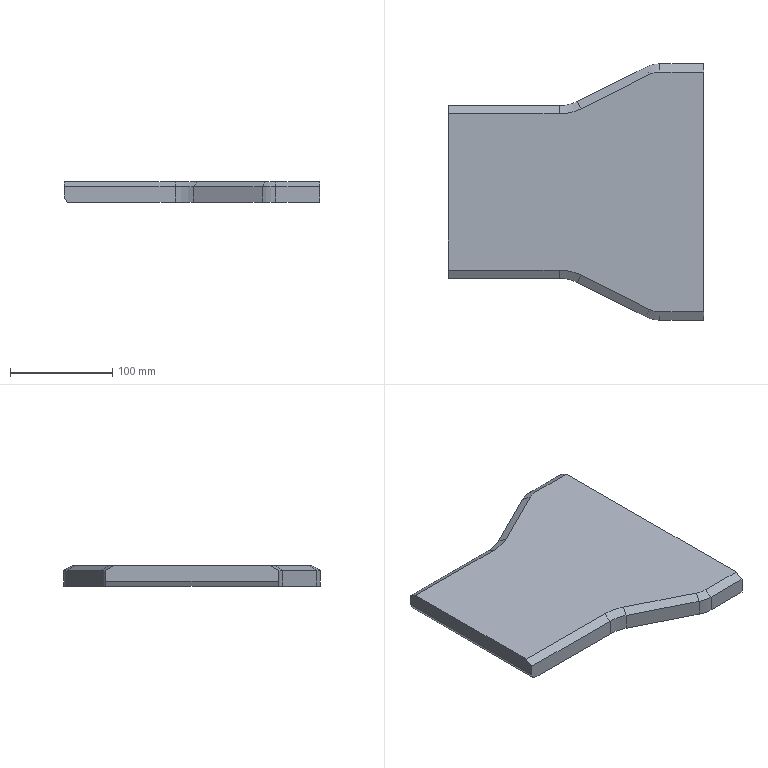Part | SolidWorks | features Chamfer 2, Extrusion 1 | 1 solid | 25 faces | box 250 x 251 x 20 mm | volume 983303 mm3 | plane 17 | cylinder 4 | cone 4 | commonest cylinder face diameters 60 x2 80 x2
STEP:
#1=CARTESIAN_POINT('',(-280.,-251.,-20.));
#2=VERTEX_POINT('',#1);
#3=CARTESIAN_POINT('',(-280.,-251.,-4.619));
#4=VERTEX_POINT('',#3);
#5=CARTESIAN_POINT('',(-280.,-251.,-20.));
#6=DIRECTION('',(0.,0.,1.));
#7=VECTOR('',#6,1000.);
#8=LINE('',#5,#7);
#9=EDGE_CURVE('',#2,#4,#8,.T.);
#10=ORIENTED_EDGE('',*,*,#9,.T.);
#11=CARTESIAN_POINT('',(-322.918,-251.,-4.619));
#12=VERTEX_POINT('',#11);
#13=CARTESIAN_POINT('',(-305.508,-251.,-4.619));
#14=DIRECTION('',(-1.,0.,0.));
#15=VECTOR('',#14,1000.);
#16=LINE('',#13,#15);
#17=EDGE_CURVE('',#4,#12,#16,.T.);
#18=ORIENTED_EDGE('',*,*,#17,.T.);
#19=CARTESIAN_POINT('',(-322.918,-251.,-20.));
#20=VERTEX_POINT('',#19);
#21=CARTESIAN_POINT('',(-322.918,-251.,-20.));
#22=DIRECTION('',(0.,0.,1.));
#23=VECTOR('',#22,1000.);
#24=LINE('',#21,#23);
#25=EDGE_CURVE('',#20,#12,#24,.T.);
#26=ORIENTED_EDGE('',*,*,#25,.F.);
#27=CARTESIAN_POINT('',(-280.,-251.,-20.));
#28=DIRECTION('',(1.,0.,0.));
#29=VECTOR('',#28,1000.);
#30=LINE('',#27,#29);
#31=EDGE_CURVE('',#20,#2,#30,.T.);
#32=ORIENTED_EDGE('',*,*,#31,.T.);
#33=EDGE_LOOP('',(#10,#18,#26,#32));
#34=FACE_OUTER_BOUND('',#33,.T.);
#35=CARTESIAN_POINT('',(-305.508,-251.,-20.));
#36=DIRECTION('',(0.,-1.,0.));
#37=DIRECTION('',(0.,0.,-1.));
#38=AXIS2_PLACEMENT_3D('',#35,#36,#37);
#39=PLANE('',#38);
#40=ADVANCED_FACE('',(#34),#39,.T.);
#41=ORIENTED_EDGE('',*,*,#25,.T.);
#42=CARTESIAN_POINT('',(-336.334,-247.833,-4.619));
#43=VERTEX_POINT('',#42);
#44=CARTESIAN_POINT('',(-322.918,-221.,-4.619));
#45=DIRECTION('',(0.,0.,-1.));
#46=DIRECTION('',(1.,0.,0.));
#47=AXIS2_PLACEMENT_3D('',#44,#45,#46);
#48=CIRCLE('',#47,30.);
#49=EDGE_CURVE('',#12,#43,#48,.T.);
#50=ORIENTED_EDGE('',*,*,#49,.T.);
#51=CARTESIAN_POINT('',(-336.334,-247.833,-20.));
#52=VERTEX_POINT('',#51);
#53=CARTESIAN_POINT('',(-336.334,-247.833,-20.));
#54=DIRECTION('',(0.,0.,1.));
#55=VECTOR('',#54,1000.);
#56=LINE('',#53,#55);
#57=EDGE_CURVE('',#52,#43,#56,.T.);
#58=ORIENTED_EDGE('',*,*,#57,.F.);
#59=CARTESIAN_POINT('',(-322.918,-221.,-20.));
#60=DIRECTION('',(0.,0.,1.));
#61=DIRECTION('',(1.,0.,0.));
#62=AXIS2_PLACEMENT_3D('',#59,#60,#61);
#63=CIRCLE('',#62,30.);
#64=EDGE_CURVE('',#52,#20,#63,.T.);
#65=ORIENTED_EDGE('',*,*,#64,.T.);
#66=EDGE_LOOP('',(#41,#50,#58,#65));
#67=FACE_OUTER_BOUND('',#66,.T.);
#68=CARTESIAN_POINT('',(-322.918,-221.,-20.));
#69=DIRECTION('',(0.,0.,1.));
#70=DIRECTION('',(1.,0.,0.));
#71=AXIS2_PLACEMENT_3D('',#68,#69,#70);
#72=CYLINDRICAL_SURFACE('',#71,30.);
#73=ADVANCED_FACE('',(#67),#72,.T.);
#74=ORIENTED_EDGE('',*,*,#57,.T.);
#75=CARTESIAN_POINT('',(-403.666,-214.167,-4.619));
#76=VERTEX_POINT('',#75);
#77=CARTESIAN_POINT('',(-403.666,-214.167,-4.619));
#78=DIRECTION('',(-0.8944,0.4472,0.));
#79=VECTOR('',#78,1000.);
#80=LINE('',#77,#79);
#81=EDGE_CURVE('',#43,#76,#80,.T.);
#82=ORIENTED_EDGE('',*,*,#81,.T.);
#83=CARTESIAN_POINT('',(-403.666,-214.167,-20.));
#84=VERTEX_POINT('',#83);
#85=CARTESIAN_POINT('',(-403.666,-214.167,-20.));
#86=DIRECTION('',(0.,0.,1.));
#87=VECTOR('',#86,1000.);
#88=LINE('',#85,#87);
#89=EDGE_CURVE('',#84,#76,#88,.T.);
#90=ORIENTED_EDGE('',*,*,#89,.F.);
#91=CARTESIAN_POINT('',(-403.666,-214.167,-20.));
#92=DIRECTION('',(0.8944,-0.4472,0.));
#93=VECTOR('',#92,1000.);
#94=LINE('',#91,#93);
#95=EDGE_CURVE('',#84,#52,#94,.T.);
#96=ORIENTED_EDGE('',*,*,#95,.T.);
#97=EDGE_LOOP('',(#74,#82,#90,#96));
#98=FACE_OUTER_BOUND('',#97,.T.);
#99=CARTESIAN_POINT('',(-403.666,-214.167,-20.));
#100=DIRECTION('',(-0.4472,-0.8944,0.));
#101=DIRECTION('',(0.8944,-0.4472,0.));
#102=AXIS2_PLACEMENT_3D('',#99,#100,#101);
#103=PLANE('',#102);
#104=ADVANCED_FACE('',(#98),#103,.T.);
#105=ORIENTED_EDGE('',*,*,#89,.T.);
#106=CARTESIAN_POINT('',(-421.554,-209.944,-4.619));
#107=VERTEX_POINT('',#106);
#108=CARTESIAN_POINT('',(-421.554,-249.944,-4.619));
#109=DIRECTION('',(0.,0.,1.));
#110=DIRECTION('',(1.,0.,0.));
#111=AXIS2_PLACEMENT_3D('',#108,#109,#110);
#112=CIRCLE('',#111,40.);
#113=EDGE_CURVE('',#76,#107,#112,.T.);
#114=ORIENTED_EDGE('',*,*,#113,.T.);
#115=CARTESIAN_POINT('',(-421.554,-209.944,-20.));
#116=VERTEX_POINT('',#115);
#117=CARTESIAN_POINT('',(-421.554,-209.944,-20.));
#118=DIRECTION('',(0.,0.,1.));
#119=VECTOR('',#118,1000.);
#120=LINE('',#117,#119);
#121=EDGE_CURVE('',#116,#107,#120,.T.);
#122=ORIENTED_EDGE('',*,*,#121,.F.);
#123=CARTESIAN_POINT('',(-421.554,-249.944,-20.));
#124=DIRECTION('',(0.,0.,-1.));
#125=DIRECTION('',(1.,0.,0.));
#126=AXIS2_PLACEMENT_3D('',#123,#124,#125);
#127=CIRCLE('',#126,40.);
#128=EDGE_CURVE('',#116,#84,#127,.T.);
#129=ORIENTED_EDGE('',*,*,#128,.T.);
#130=EDGE_LOOP('',(#105,#114,#122,#129));
#131=FACE_OUTER_BOUND('',#130,.T.);
#132=CARTESIAN_POINT('',(-421.554,-249.944,-20.));
#133=DIRECTION('',(0.,0.,1.));
#134=DIRECTION('',(1.,0.,0.));
#135=AXIS2_PLACEMENT_3D('',#132,#133,#134);
#136=CYLINDRICAL_SURFACE('',#135,40.);
#137=ADVANCED_FACE('',(#131),#136,.F.);
#138=CARTESIAN_POINT('',(-530.,-209.944,-15.));
#139=VERTEX_POINT('',#138);
#140=CARTESIAN_POINT('',(-530.,-209.944,-4.619));
#141=VERTEX_POINT('',#140);
#142=CARTESIAN_POINT('',(-530.,-209.944,-20.));
#143=DIRECTION('',(0.,0.,1.));
#144=VECTOR('',#143,1000.);
#145=LINE('',#142,#144);
#146=EDGE_CURVE('',#139,#141,#145,.T.);
#147=ORIENTED_EDGE('',*,*,#146,.F.);
#148=CARTESIAN_POINT('',(-527.113,-209.944,-20.));
#149=VERTEX_POINT('',#148);
#150=CARTESIAN_POINT('',(-500.723,-209.944,-65.708));
#151=DIRECTION('',(0.5,0.,-0.866));
#152=VECTOR('',#151,1000.);
#153=LINE('',#150,#152);
#154=EDGE_CURVE('',#139,#149,#153,.T.);
#155=ORIENTED_EDGE('',*,*,#154,.T.);
#156=CARTESIAN_POINT('',(-421.554,-209.944,-20.));
#157=DIRECTION('',(1.,0.,0.));
#158=VECTOR('',#157,1000.);
#159=LINE('',#156,#158);
#160=EDGE_CURVE('',#149,#116,#159,.T.);
#161=ORIENTED_EDGE('',*,*,#160,.T.);
#162=ORIENTED_EDGE('',*,*,#121,.T.);
#163=CARTESIAN_POINT('',(-421.554,-209.944,-4.619));
#164=DIRECTION('',(-1.,0.,0.));
#165=VECTOR('',#164,1000.);
#166=LINE('',#163,#165);
#167=EDGE_CURVE('',#107,#141,#166,.T.);
#168=ORIENTED_EDGE('',*,*,#167,.T.);
#169=EDGE_LOOP('',(#147,#155,#161,#162,#168));
#170=FACE_OUTER_BOUND('',#169,.T.);
#171=CARTESIAN_POINT('',(-421.554,-209.944,-20.));
#172=DIRECTION('',(0.,-1.,0.));
#173=DIRECTION('',(0.,0.,-1.));
#174=AXIS2_PLACEMENT_3D('',#171,#172,#173);
#175=PLANE('',#174);
#176=ADVANCED_FACE('',(#170),#175,.T.);
#177=CARTESIAN_POINT('',(-530.,-41.056,-15.));
#178=VERTEX_POINT('',#177);
#179=CARTESIAN_POINT('',(-530.,-41.056,-4.619));
#180=VERTEX_POINT('',#179);
#181=CARTESIAN_POINT('',(-530.,-41.056,-20.));
#182=DIRECTION('',(0.,0.,1.));
#183=VECTOR('',#182,1000.);
#184=LINE('',#181,#183);
#185=EDGE_CURVE('',#178,#180,#184,.T.);
#186=ORIENTED_EDGE('',*,*,#185,.F.);
#187=CARTESIAN_POINT('',(-530.,-209.944,-15.));
#188=DIRECTION('',(0.,-1.,0.));
#189=VECTOR('',#188,1000.);
#190=LINE('',#187,#189);
#191=EDGE_CURVE('',#178,#139,#190,.T.);
#192=ORIENTED_EDGE('',*,*,#191,.T.);
#193=ORIENTED_EDGE('',*,*,#146,.T.);
#194=CARTESIAN_POINT('',(-530.,-201.944,0.));
#195=VERTEX_POINT('',#194);
#196=CARTESIAN_POINT('',(-530.,-89.938,64.667));
#197=DIRECTION('',(0.,0.866,0.5));
#198=VECTOR('',#197,1000.);
#199=LINE('',#196,#198);
#200=EDGE_CURVE('',#141,#195,#199,.T.);
#201=ORIENTED_EDGE('',*,*,#200,.T.);
#202=CARTESIAN_POINT('',(-530.,-49.056,0.));
#203=VERTEX_POINT('',#202);
#204=CARTESIAN_POINT('',(-530.,-41.056,0.));
#205=DIRECTION('',(0.,-1.,0.));
#206=VECTOR('',#205,1000.);
#207=LINE('',#204,#206);
#208=EDGE_CURVE('',#203,#195,#207,.T.);
#209=ORIENTED_EDGE('',*,*,#208,.F.);
#210=CARTESIAN_POINT('',(-530.,-34.395,-8.464));
#211=DIRECTION('',(0.,0.866,-0.5));
#212=VECTOR('',#211,1000.);
#213=LINE('',#210,#212);
#214=EDGE_CURVE('',#203,#180,#213,.T.);
#215=ORIENTED_EDGE('',*,*,#214,.T.);
#216=EDGE_LOOP('',(#186,#192,#193,#201,#209,#215));
#217=FACE_OUTER_BOUND('',#216,.T.);
#218=CARTESIAN_POINT('',(-530.,-41.056,-20.));
#219=DIRECTION('',(-1.,0.,0.));
#220=DIRECTION('',(0.,0.,1.));
#221=AXIS2_PLACEMENT_3D('',#218,#219,#220);
#222=PLANE('',#221);
#223=ADVANCED_FACE('',(#217),#222,.T.);
#224=CARTESIAN_POINT('',(-421.554,-41.056,-20.));
#225=VERTEX_POINT('',#224);
#226=CARTESIAN_POINT('',(-527.113,-41.056,-20.));
#227=VERTEX_POINT('',#226);
#228=CARTESIAN_POINT('',(-530.,-41.056,-20.));
#229=DIRECTION('',(-1.,0.,0.));
#230=VECTOR('',#229,1000.);
#231=LINE('',#228,#230);
#232=EDGE_CURVE('',#225,#227,#231,.T.);
#233=ORIENTED_EDGE('',*,*,#232,.T.);
#234=CARTESIAN_POINT('',(-527.835,-41.056,-18.75));
#235=DIRECTION('',(-0.5,0.,0.866));
#236=VECTOR('',#235,1000.);
#237=LINE('',#234,#236);
#238=EDGE_CURVE('',#227,#178,#237,.T.);
#239=ORIENTED_EDGE('',*,*,#238,.T.);
#240=ORIENTED_EDGE('',*,*,#185,.T.);
#241=CARTESIAN_POINT('',(-421.554,-41.056,-4.619));
#242=VERTEX_POINT('',#241);
#243=CARTESIAN_POINT('',(-530.,-41.056,-4.619));
#244=DIRECTION('',(1.,0.,0.));
#245=VECTOR('',#244,1000.);
#246=LINE('',#243,#245);
#247=EDGE_CURVE('',#180,#242,#246,.T.);
#248=ORIENTED_EDGE('',*,*,#247,.T.);
#249=CARTESIAN_POINT('',(-421.554,-41.056,-20.));
#250=DIRECTION('',(0.,0.,1.));
#251=VECTOR('',#250,1000.);
#252=LINE('',#249,#251);
#253=EDGE_CURVE('',#225,#242,#252,.T.);
#254=ORIENTED_EDGE('',*,*,#253,.F.);
#255=EDGE_LOOP('',(#233,#239,#240,#248,#254));
#256=FACE_OUTER_BOUND('',#255,.T.);
#257=CARTESIAN_POINT('',(-530.,-41.056,-20.));
#258=DIRECTION('',(0.,1.,0.));
#259=DIRECTION('',(-1.,0.,0.));
#260=AXIS2_PLACEMENT_3D('',#257,#258,#259);
#261=PLANE('',#260);
#262=ADVANCED_FACE('',(#256),#261,.T.);
#263=ORIENTED_EDGE('',*,*,#253,.T.);
#264=CARTESIAN_POINT('',(-403.666,-36.833,-4.619));
#265=VERTEX_POINT('',#264);
#266=CARTESIAN_POINT('',(-421.554,-1.056,-4.619));
#267=DIRECTION('',(0.,0.,1.));
#268=DIRECTION('',(1.,0.,0.));
#269=AXIS2_PLACEMENT_3D('',#266,#267,#268);
#270=CIRCLE('',#269,40.);
#271=EDGE_CURVE('',#242,#265,#270,.T.);
#272=ORIENTED_EDGE('',*,*,#271,.T.);
#273=CARTESIAN_POINT('',(-403.666,-36.833,-20.));
#274=VERTEX_POINT('',#273);
#275=CARTESIAN_POINT('',(-403.666,-36.833,-20.));
#276=DIRECTION('',(0.,0.,1.));
#277=VECTOR('',#276,1000.);
#278=LINE('',#275,#277);
#279=EDGE_CURVE('',#274,#265,#278,.T.);
#280=ORIENTED_EDGE('',*,*,#279,.F.);
#281=CARTESIAN_POINT('',(-421.554,-1.056,-20.));
#282=DIRECTION('',(0.,0.,-1.));
#283=DIRECTION('',(1.,0.,0.));
#284=AXIS2_PLACEMENT_3D('',#281,#282,#283);
#285=CIRCLE('',#284,40.);
#286=EDGE_CURVE('',#274,#225,#285,.T.);
#287=ORIENTED_EDGE('',*,*,#286,.T.);
#288=EDGE_LOOP('',(#263,#272,#280,#287));
#289=FACE_OUTER_BOUND('',#288,.T.);
#290=CARTESIAN_POINT('',(-421.554,-1.056,-20.));
#291=DIRECTION('',(0.,0.,1.));
#292=DIRECTION('',(1.,0.,0.));
#293=AXIS2_PLACEMENT_3D('',#290,#291,#292);
#294=CYLINDRICAL_SURFACE('',#293,40.);
#295=ADVANCED_FACE('',(#289),#294,.F.);
#296=ORIENTED_EDGE('',*,*,#279,.T.);
#297=CARTESIAN_POINT('',(-336.334,-3.167,-4.619));
#298=VERTEX_POINT('',#297);
#299=CARTESIAN_POINT('',(-403.666,-36.833,-4.619));
#300=DIRECTION('',(0.8944,0.4472,0.));
#301=VECTOR('',#300,1000.);
#302=LINE('',#299,#301);
#303=EDGE_CURVE('',#265,#298,#302,.T.);
#304=ORIENTED_EDGE('',*,*,#303,.T.);
#305=CARTESIAN_POINT('',(-336.334,-3.167,-20.));
#306=VERTEX_POINT('',#305);
#307=CARTESIAN_POINT('',(-336.334,-3.167,-20.));
#308=DIRECTION('',(0.,0.,1.));
#309=VECTOR('',#308,1000.);
#310=LINE('',#307,#309);
#311=EDGE_CURVE('',#306,#298,#310,.T.);
#312=ORIENTED_EDGE('',*,*,#311,.F.);
#313=CARTESIAN_POINT('',(-403.666,-36.833,-20.));
#314=DIRECTION('',(-0.8944,-0.4472,0.));
#315=VECTOR('',#314,1000.);
#316=LINE('',#313,#315);
#317=EDGE_CURVE('',#306,#274,#316,.T.);
#318=ORIENTED_EDGE('',*,*,#317,.T.);
#319=EDGE_LOOP('',(#296,#304,#312,#318));
#320=FACE_OUTER_BOUND('',#319,.T.);
#321=CARTESIAN_POINT('',(-403.666,-36.833,-20.));
#322=DIRECTION('',(-0.4472,0.8944,0.));
#323=DIRECTION('',(-0.8944,-0.4472,0.));
#324=AXIS2_PLACEMENT_3D('',#321,#322,#323);
#325=PLANE('',#324);
#326=ADVANCED_FACE('',(#320),#325,.T.);
#327=ORIENTED_EDGE('',*,*,#311,.T.);
#328=CARTESIAN_POINT('',(-322.918,0.,-4.619));
#329=VERTEX_POINT('',#328);
#330=CARTESIAN_POINT('',(-322.918,-30.,-4.619));
#331=DIRECTION('',(0.,0.,-1.));
#332=DIRECTION('',(1.,0.,0.));
#333=AXIS2_PLACEMENT_3D('',#330,#331,#332);
#334=CIRCLE('',#333,30.);
#335=EDGE_CURVE('',#298,#329,#334,.T.);
#336=ORIENTED_EDGE('',*,*,#335,.T.);
#337=CARTESIAN_POINT('',(-322.918,0.,-20.));
#338=VERTEX_POINT('',#337);
#339=CARTESIAN_POINT('',(-322.918,0.,-20.));
#340=DIRECTION('',(0.,0.,1.));
#341=VECTOR('',#340,1000.);
#342=LINE('',#339,#341);
#343=EDGE_CURVE('',#338,#329,#342,.T.);
#344=ORIENTED_EDGE('',*,*,#343,.F.);
#345=CARTESIAN_POINT('',(-322.918,-30.,-20.));
#346=DIRECTION('',(0.,0.,1.));
#347=DIRECTION('',(1.,0.,0.));
#348=AXIS2_PLACEMENT_3D('',#345,#346,#347);
#349=CIRCLE('',#348,30.);
#350=EDGE_CURVE('',#338,#306,#349,.T.);
#351=ORIENTED_EDGE('',*,*,#350,.T.);
#352=EDGE_LOOP('',(#327,#336,#344,#351));
#353=FACE_OUTER_BOUND('',#352,.T.);
#354=CARTESIAN_POINT('',(-322.918,-30.,-20.));
#355=DIRECTION('',(0.,0.,1.));
#356=DIRECTION('',(1.,0.,0.));
#357=AXIS2_PLACEMENT_3D('',#354,#355,#356);
#358=CYLINDRICAL_SURFACE('',#357,30.);
#359=ADVANCED_FACE('',(#353),#358,.T.);
#360=ORIENTED_EDGE('',*,*,#343,.T.);
#361=CARTESIAN_POINT('',(-280.,0.,-4.619));
#362=VERTEX_POINT('',#361);
#363=CARTESIAN_POINT('',(-300.,0.,-4.619));
#364=DIRECTION('',(1.,0.,0.));
#365=VECTOR('',#364,1000.);
#366=LINE('',#363,#365);
#367=EDGE_CURVE('',#329,#362,#366,.T.);
#368=ORIENTED_EDGE('',*,*,#367,.T.);
#369=CARTESIAN_POINT('',(-280.,0.,-20.));
#370=VERTEX_POINT('',#369);
#371=CARTESIAN_POINT('',(-280.,0.,-20.));
#372=DIRECTION('',(0.,0.,1.));
#373=VECTOR('',#372,1000.);
#374=LINE('',#371,#373);
#375=EDGE_CURVE('',#370,#362,#374,.T.);
#376=ORIENTED_EDGE('',*,*,#375,.F.);
#377=CARTESIAN_POINT('',(-300.,0.,-20.));
#378=DIRECTION('',(-1.,0.,0.));
#379=VECTOR('',#378,1000.);
#380=LINE('',#377,#379);
#381=EDGE_CURVE('',#370,#338,#380,.T.);
#382=ORIENTED_EDGE('',*,*,#381,.T.);
#383=EDGE_LOOP('',(#360,#368,#376,#382));
#384=FACE_OUTER_BOUND('',#383,.T.);
#385=CARTESIAN_POINT('',(-300.,0.,-20.));
#386=DIRECTION('',(0.,1.,0.));
#387=DIRECTION('',(0.,0.,1.));
#388=AXIS2_PLACEMENT_3D('',#385,#386,#387);
#389=PLANE('',#388);
#390=ADVANCED_FACE('',(#384),#389,.T.);
#391=CARTESIAN_POINT('',(-280.,-243.,0.));
#392=VERTEX_POINT('',#391);
#393=CARTESIAN_POINT('',(-280.,-8.,0.));
#394=VERTEX_POINT('',#393);
#395=CARTESIAN_POINT('',(-280.,0.,0.));
#396=DIRECTION('',(0.,1.,0.));
#397=VECTOR('',#396,1000.);
#398=LINE('',#395,#397);
#399=EDGE_CURVE('',#392,#394,#398,.T.);
#400=ORIENTED_EDGE('',*,*,#399,.F.);
#401=CARTESIAN_POINT('',(-280.,-69.41,100.222));
#402=DIRECTION('',(0.,-0.866,-0.5));
#403=VECTOR('',#402,1000.);
#404=LINE('',#401,#403);
#405=EDGE_CURVE('',#392,#4,#404,.T.);
#406=ORIENTED_EDGE('',*,*,#405,.T.);
#407=ORIENTED_EDGE('',*,*,#9,.F.);
#408=CARTESIAN_POINT('',(-280.,0.,-20.));
#409=DIRECTION('',(0.,1.,0.));
#410=VECTOR('',#409,1000.);
#411=LINE('',#408,#410);
#412=EDGE_CURVE('',#2,#370,#411,.T.);
#413=ORIENTED_EDGE('',*,*,#412,.T.);
#414=ORIENTED_EDGE('',*,*,#375,.T.);
#415=CARTESIAN_POINT('',(-280.,6.66,-8.464));
#416=DIRECTION('',(0.,-0.866,0.5));
#417=VECTOR('',#416,1000.);
#418=LINE('',#415,#417);
#419=EDGE_CURVE('',#362,#394,#418,.T.);
#420=ORIENTED_EDGE('',*,*,#419,.T.);
#421=EDGE_LOOP('',(#400,#406,#407,#413,#414,#420));
#422=FACE_OUTER_BOUND('',#421,.T.);
#423=CARTESIAN_POINT('',(-280.,0.,-20.));
#424=DIRECTION('',(1.,0.,0.));
#425=DIRECTION('',(0.,1.,0.));
#426=AXIS2_PLACEMENT_3D('',#423,#424,#425);
#427=PLANE('',#426);
#428=ADVANCED_FACE('',(#422),#427,.T.);
#429=ORIENTED_EDGE('',*,*,#160,.F.);
#430=CARTESIAN_POINT('',(-527.113,-41.056,-20.));
#431=DIRECTION('',(0.,1.,0.));
#432=VECTOR('',#431,1000.);
#433=LINE('',#430,#432);
#434=EDGE_CURVE('',#149,#227,#433,.T.);
#435=ORIENTED_EDGE('',*,*,#434,.T.);
#436=ORIENTED_EDGE('',*,*,#232,.F.);
#437=ORIENTED_EDGE('',*,*,#286,.F.);
#438=ORIENTED_EDGE('',*,*,#317,.F.);
#439=ORIENTED_EDGE('',*,*,#350,.F.);
#440=ORIENTED_EDGE('',*,*,#381,.F.);
#441=ORIENTED_EDGE('',*,*,#412,.F.);
#442=ORIENTED_EDGE('',*,*,#31,.F.);
#443=ORIENTED_EDGE('',*,*,#64,.F.);
#444=ORIENTED_EDGE('',*,*,#95,.F.);
#445=ORIENTED_EDGE('',*,*,#128,.F.);
#446=EDGE_LOOP('',(#429,#435,#436,#437,#438,#439,#440,#441,#442,#443,#444,#445));
#447=FACE_OUTER_BOUND('',#446,.T.);
#448=CARTESIAN_POINT('',(-322.918,-221.,-20.));
#449=DIRECTION('',(0.,0.,1.));
#450=DIRECTION('',(1.,0.,0.));
#451=AXIS2_PLACEMENT_3D('',#448,#449,#450);
#452=PLANE('',#451);
#453=ADVANCED_FACE('',(#447),#452,.F.);
#454=ORIENTED_EDGE('',*,*,#208,.T.);
#455=CARTESIAN_POINT('',(-421.554,-201.944,0.));
#456=VERTEX_POINT('',#455);
#457=CARTESIAN_POINT('',(-322.918,-201.944,0.));
#458=DIRECTION('',(1.,0.,0.));
#459=VECTOR('',#458,1000.);
#460=LINE('',#457,#459);
#461=EDGE_CURVE('',#195,#456,#460,.T.);
#462=ORIENTED_EDGE('',*,*,#461,.T.);
#463=CARTESIAN_POINT('',(-400.088,-207.012,0.));
#464=VERTEX_POINT('',#463);
#465=CARTESIAN_POINT('',(-421.554,-249.944,0.));
#466=DIRECTION('',(0.,0.,-1.));
#467=DIRECTION('',(1.,0.,0.));
#468=AXIS2_PLACEMENT_3D('',#465,#466,#467);
#469=CIRCLE('',#468,48.);
#470=EDGE_CURVE('',#456,#464,#469,.T.);
#471=ORIENTED_EDGE('',*,*,#470,.T.);
#472=CARTESIAN_POINT('',(-332.757,-240.677,0.));
#473=VERTEX_POINT('',#472);
#474=CARTESIAN_POINT('',(-332.757,-240.677,0.));
#475=DIRECTION('',(0.8944,-0.4472,0.));
#476=VECTOR('',#475,1000.);
#477=LINE('',#474,#476);
#478=EDGE_CURVE('',#464,#473,#477,.T.);
#479=ORIENTED_EDGE('',*,*,#478,.T.);
#480=CARTESIAN_POINT('',(-322.918,-243.,0.));
#481=VERTEX_POINT('',#480);
#482=CARTESIAN_POINT('',(-322.918,-221.,0.));
#483=DIRECTION('',(0.,0.,1.));
#484=DIRECTION('',(1.,0.,0.));
#485=AXIS2_PLACEMENT_3D('',#482,#483,#484);
#486=CIRCLE('',#485,22.);
#487=EDGE_CURVE('',#473,#481,#486,.T.);
#488=ORIENTED_EDGE('',*,*,#487,.T.);
#489=CARTESIAN_POINT('',(-322.918,-243.,0.));
#490=DIRECTION('',(1.,0.,0.));
#491=VECTOR('',#490,1000.);
#492=LINE('',#489,#491);
#493=EDGE_CURVE('',#481,#392,#492,.T.);
#494=ORIENTED_EDGE('',*,*,#493,.T.);
#495=ORIENTED_EDGE('',*,*,#399,.T.);
#496=CARTESIAN_POINT('',(-322.918,-8.,0.));
#497=VERTEX_POINT('',#496);
#498=CARTESIAN_POINT('',(-322.918,-8.,0.));
#499=DIRECTION('',(-1.,0.,0.));
#500=VECTOR('',#499,1000.);
#501=LINE('',#498,#500);
#502=EDGE_CURVE('',#394,#497,#501,.T.);
#503=ORIENTED_EDGE('',*,*,#502,.T.);
#504=CARTESIAN_POINT('',(-332.757,-10.323,0.));
#505=VERTEX_POINT('',#504);
#506=CARTESIAN_POINT('',(-322.918,-30.,0.));
#507=DIRECTION('',(0.,0.,1.));
#508=DIRECTION('',(1.,0.,0.));
#509=AXIS2_PLACEMENT_3D('',#506,#507,#508);
#510=CIRCLE('',#509,22.);
#511=EDGE_CURVE('',#497,#505,#510,.T.);
#512=ORIENTED_EDGE('',*,*,#511,.T.);
#513=CARTESIAN_POINT('',(-400.088,-43.988,0.));
#514=VERTEX_POINT('',#513);
#515=CARTESIAN_POINT('',(-409.157,-48.523,0.));
#516=DIRECTION('',(-0.8944,-0.4472,0.));
#517=VECTOR('',#516,1000.);
#518=LINE('',#515,#517);
#519=EDGE_CURVE('',#505,#514,#518,.T.);
#520=ORIENTED_EDGE('',*,*,#519,.T.);
#521=CARTESIAN_POINT('',(-421.554,-49.056,0.));
#522=VERTEX_POINT('',#521);
#523=CARTESIAN_POINT('',(-421.554,-1.056,0.));
#524=DIRECTION('',(0.,0.,-1.));
#525=DIRECTION('',(1.,0.,0.));
#526=AXIS2_PLACEMENT_3D('',#523,#524,#525);
#527=CIRCLE('',#526,48.);
#528=EDGE_CURVE('',#514,#522,#527,.T.);
#529=ORIENTED_EDGE('',*,*,#528,.T.);
#530=CARTESIAN_POINT('',(-322.918,-49.056,0.));
#531=DIRECTION('',(-1.,0.,0.));
#532=VECTOR('',#531,1000.);
#533=LINE('',#530,#532);
#534=EDGE_CURVE('',#522,#203,#533,.T.);
#535=ORIENTED_EDGE('',*,*,#534,.T.);
#536=EDGE_LOOP('',(#454,#462,#471,#479,#488,#494,#495,#503,#512,#520,#529,#535));
#537=FACE_OUTER_BOUND('',#536,.T.);
#538=CARTESIAN_POINT('',(-322.918,-221.,0.));
#539=DIRECTION('',(0.,0.,1.));
#540=DIRECTION('',(1.,0.,0.));
#541=AXIS2_PLACEMENT_3D('',#538,#539,#540);
#542=PLANE('',#541);
#543=ADVANCED_FACE('',(#537),#542,.T.);
#544=ORIENTED_EDGE('',*,*,#419,.F.);
#545=ORIENTED_EDGE('',*,*,#367,.F.);
#546=CARTESIAN_POINT('',(-322.918,-8.,0.));
#547=DIRECTION('',(0.,0.866,-0.5));
#548=VECTOR('',#547,1000.);
#549=LINE('',#546,#548);
#550=EDGE_CURVE('',#497,#329,#549,.T.);
#551=ORIENTED_EDGE('',*,*,#550,.F.);
#552=ORIENTED_EDGE('',*,*,#502,.F.);
#553=EDGE_LOOP('',(#544,#545,#551,#552));
#554=FACE_OUTER_BOUND('',#553,.T.);
#555=CARTESIAN_POINT('',(-322.918,-8.,0.));
#556=DIRECTION('',(0.,-0.5,-0.866));
#557=DIRECTION('',(-1.,0.,0.));
#558=AXIS2_PLACEMENT_3D('',#555,#556,#557);
#559=PLANE('',#558);
#560=ADVANCED_FACE('',(#554),#559,.F.);
#561=ORIENTED_EDGE('',*,*,#214,.F.);
#562=ORIENTED_EDGE('',*,*,#534,.F.);
#563=CARTESIAN_POINT('',(-421.554,-41.056,-4.619));
#564=DIRECTION('',(0.,-0.866,0.5));
#565=VECTOR('',#564,1000.);
#566=LINE('',#563,#565);
#567=EDGE_CURVE('',#242,#522,#566,.T.);
#568=ORIENTED_EDGE('',*,*,#567,.F.);
#569=ORIENTED_EDGE('',*,*,#247,.F.);
#570=EDGE_LOOP('',(#561,#562,#568,#569));
#571=FACE_OUTER_BOUND('',#570,.T.);
#572=CARTESIAN_POINT('',(-322.918,-49.056,0.));
#573=DIRECTION('',(0.,-0.5,-0.866));
#574=DIRECTION('',(-1.,0.,0.));
#575=AXIS2_PLACEMENT_3D('',#572,#573,#574);
#576=PLANE('',#575);
#577=ADVANCED_FACE('',(#571),#576,.F.);
#578=ORIENTED_EDGE('',*,*,#550,.T.);
#579=ORIENTED_EDGE('',*,*,#335,.F.);
#580=CARTESIAN_POINT('',(-332.757,-10.323,0.));
#581=DIRECTION('',(-0.3873,0.7746,-0.5));
#582=VECTOR('',#581,1000.);
#583=LINE('',#580,#582);
#584=EDGE_CURVE('',#505,#298,#583,.T.);
#585=ORIENTED_EDGE('',*,*,#584,.F.);
#586=ORIENTED_EDGE('',*,*,#511,.F.);
#587=EDGE_LOOP('',(#578,#579,#585,#586));
#588=FACE_OUTER_BOUND('',#587,.T.);
#589=CARTESIAN_POINT('',(-322.918,-30.,0.));
#590=DIRECTION('',(0.,0.,-1.));
#591=DIRECTION('',(-1.,0.,0.));
#592=AXIS2_PLACEMENT_3D('',#589,#590,#591);
#593=CONICAL_SURFACE('',#592,22.,1.047);
#594=ADVANCED_FACE('',(#588),#593,.T.);
#595=ORIENTED_EDGE('',*,*,#567,.T.);
#596=ORIENTED_EDGE('',*,*,#528,.F.);
#597=CARTESIAN_POINT('',(-403.666,-36.833,-4.619));
#598=DIRECTION('',(0.3873,-0.7746,0.5));
#599=VECTOR('',#598,1000.);
#600=LINE('',#597,#599);
#601=EDGE_CURVE('',#265,#514,#600,.T.);
#602=ORIENTED_EDGE('',*,*,#601,.F.);
#603=ORIENTED_EDGE('',*,*,#271,.F.);
#604=EDGE_LOOP('',(#595,#596,#602,#603));
#605=FACE_OUTER_BOUND('',#604,.T.);
#606=CARTESIAN_POINT('',(-421.554,-1.056,0.));
#607=DIRECTION('',(0.,0.,1.));
#608=DIRECTION('',(1.,0.,0.));
#609=AXIS2_PLACEMENT_3D('',#606,#607,#608);
#610=CONICAL_SURFACE('',#609,48.,1.047);
#611=ADVANCED_FACE('',(#605),#610,.F.);
#612=ORIENTED_EDGE('',*,*,#584,.T.);
#613=ORIENTED_EDGE('',*,*,#303,.F.);
#614=ORIENTED_EDGE('',*,*,#601,.T.);
#615=ORIENTED_EDGE('',*,*,#519,.F.);
#616=EDGE_LOOP('',(#612,#613,#614,#615));
#617=FACE_OUTER_BOUND('',#616,.T.);
#618=CARTESIAN_POINT('',(-409.157,-48.523,0.));
#619=DIRECTION('',(0.2236,-0.4472,-0.866));
#620=DIRECTION('',(-0.8944,-0.4472,0.));
#621=AXIS2_PLACEMENT_3D('',#618,#619,#620);
#622=PLANE('',#621);
#623=ADVANCED_FACE('',(#617),#622,.F.);
#624=ORIENTED_EDGE('',*,*,#405,.F.);
#625=ORIENTED_EDGE('',*,*,#493,.F.);
#626=CARTESIAN_POINT('',(-322.918,-251.,-4.619));
#627=DIRECTION('',(0.,0.866,0.5));
#628=VECTOR('',#627,1000.);
#629=LINE('',#626,#628);
#630=EDGE_CURVE('',#12,#481,#629,.T.);
#631=ORIENTED_EDGE('',*,*,#630,.F.);
#632=ORIENTED_EDGE('',*,*,#17,.F.);
#633=EDGE_LOOP('',(#624,#625,#631,#632));
#634=FACE_OUTER_BOUND('',#633,.T.);
#635=CARTESIAN_POINT('',(-322.918,-243.,0.));
#636=DIRECTION('',(0.,0.5,-0.866));
#637=DIRECTION('',(1.,0.,0.));
#638=AXIS2_PLACEMENT_3D('',#635,#636,#637);
#639=PLANE('',#638);
#640=ADVANCED_FACE('',(#634),#639,.F.);
#641=ORIENTED_EDGE('',*,*,#630,.T.);
#642=ORIENTED_EDGE('',*,*,#487,.F.);
#643=CARTESIAN_POINT('',(-336.334,-247.833,-4.619));
#644=DIRECTION('',(0.3873,0.7746,0.5));
#645=VECTOR('',#644,1000.);
#646=LINE('',#643,#645);
#647=EDGE_CURVE('',#43,#473,#646,.T.);
#648=ORIENTED_EDGE('',*,*,#647,.F.);
#649=ORIENTED_EDGE('',*,*,#49,.F.);
#650=EDGE_LOOP('',(#641,#642,#648,#649));
#651=FACE_OUTER_BOUND('',#650,.T.);
#652=CARTESIAN_POINT('',(-322.918,-221.,0.));
#653=DIRECTION('',(0.,0.,-1.));
#654=DIRECTION('',(-1.,0.,0.));
#655=AXIS2_PLACEMENT_3D('',#652,#653,#654);
#656=CONICAL_SURFACE('',#655,22.,1.047);
#657=ADVANCED_FACE('',(#651),#656,.T.);
#658=ORIENTED_EDGE('',*,*,#647,.T.);
#659=ORIENTED_EDGE('',*,*,#478,.F.);
#660=CARTESIAN_POINT('',(-403.666,-214.167,-4.619));
#661=DIRECTION('',(0.3873,0.7746,0.5));
#662=VECTOR('',#661,1000.);
#663=LINE('',#660,#662);
#664=EDGE_CURVE('',#76,#464,#663,.T.);
#665=ORIENTED_EDGE('',*,*,#664,.F.);
#666=ORIENTED_EDGE('',*,*,#81,.F.);
#667=EDGE_LOOP('',(#658,#659,#665,#666));
#668=FACE_OUTER_BOUND('',#667,.T.);
#669=CARTESIAN_POINT('',(-332.757,-240.677,0.));
#670=DIRECTION('',(0.2236,0.4472,-0.866));
#671=DIRECTION('',(0.8944,-0.4472,0.));
#672=AXIS2_PLACEMENT_3D('',#669,#670,#671);
#673=PLANE('',#672);
#674=ADVANCED_FACE('',(#668),#673,.F.);
#675=ORIENTED_EDGE('',*,*,#664,.T.);
#676=ORIENTED_EDGE('',*,*,#470,.F.);
#677=CARTESIAN_POINT('',(-421.554,-209.944,-4.619));
#678=DIRECTION('',(0.,0.866,0.5));
#679=VECTOR('',#678,1000.);
#680=LINE('',#677,#679);
#681=EDGE_CURVE('',#107,#456,#680,.T.);
#682=ORIENTED_EDGE('',*,*,#681,.F.);
#683=ORIENTED_EDGE('',*,*,#113,.F.);
#684=EDGE_LOOP('',(#675,#676,#682,#683));
#685=FACE_OUTER_BOUND('',#684,.T.);
#686=CARTESIAN_POINT('',(-421.554,-249.944,0.));
#687=DIRECTION('',(0.,0.,1.));
#688=DIRECTION('',(1.,0.,0.));
#689=AXIS2_PLACEMENT_3D('',#686,#687,#688);
#690=CONICAL_SURFACE('',#689,48.,1.047);
#691=ADVANCED_FACE('',(#685),#690,.F.);
#692=ORIENTED_EDGE('',*,*,#200,.F.);
#693=ORIENTED_EDGE('',*,*,#167,.F.);
#694=ORIENTED_EDGE('',*,*,#681,.T.);
#695=ORIENTED_EDGE('',*,*,#461,.F.);
#696=EDGE_LOOP('',(#692,#693,#694,#695));
#697=FACE_OUTER_BOUND('',#696,.T.);
#698=CARTESIAN_POINT('',(-322.918,-201.944,0.));
#699=DIRECTION('',(0.,0.5,-0.866));
#700=DIRECTION('',(1.,0.,0.));
#701=AXIS2_PLACEMENT_3D('',#698,#699,#700);
#702=PLANE('',#701);
#703=ADVANCED_FACE('',(#697),#702,.F.);
#704=ORIENTED_EDGE('',*,*,#238,.F.);
#705=ORIENTED_EDGE('',*,*,#434,.F.);
#706=ORIENTED_EDGE('',*,*,#154,.F.);
#707=ORIENTED_EDGE('',*,*,#191,.F.);
#708=EDGE_LOOP('',(#704,#705,#706,#707));
#709=FACE_OUTER_BOUND('',#708,.T.);
#710=CARTESIAN_POINT('',(-530.,-41.056,-15.));
#711=DIRECTION('',(-0.866,0.,-0.5));
#712=DIRECTION('',(0.,1.,0.));
#713=AXIS2_PLACEMENT_3D('',#710,#711,#712);
#714=PLANE('',#713);
#715=ADVANCED_FACE('',(#709),#714,.T.);
#716=CLOSED_SHELL('',(#40,#73,#104,#137,#176,#223,#262,#295,#326,#359,#390,#428,#453,#543,#560,#577,#594,#611,#623,#640,#657,#674,#691,#703,#715));
#717=MANIFOLD_SOLID_BREP('',#716);
#718=CARTESIAN_POINT('',(0.,0.,0.));
#719=DIRECTION('',(0.,0.,1.));
#720=DIRECTION('',(1.,0.,0.));
#721=AXIS2_PLACEMENT_3D('',#718,#719,#720);
#722=(LENGTH_UNIT()NAMED_UNIT(*)SI_UNIT(.MILLI.,.METRE.));
#723=UNCERTAINTY_MEASURE_WITH_UNIT(LENGTH_MEASURE(0.00001),#722,'','');
#724=(NAMED_UNIT(*)PLANE_ANGLE_UNIT()SI_UNIT($,.RADIAN.));
#725=(NAMED_UNIT(*)SI_UNIT($,.STERADIAN.)SOLID_ANGLE_UNIT());
#726=(GEOMETRIC_REPRESENTATION_CONTEXT(3)GLOBAL_UNCERTAINTY_ASSIGNED_CONTEXT((#723))GLOBAL_UNIT_ASSIGNED_CONTEXT((#722,#724,#725))REPRESENTATION_CONTEXT('',''));
#727=ADVANCED_BREP_SHAPE_REPRESENTATION('',(#717,#721),#726);